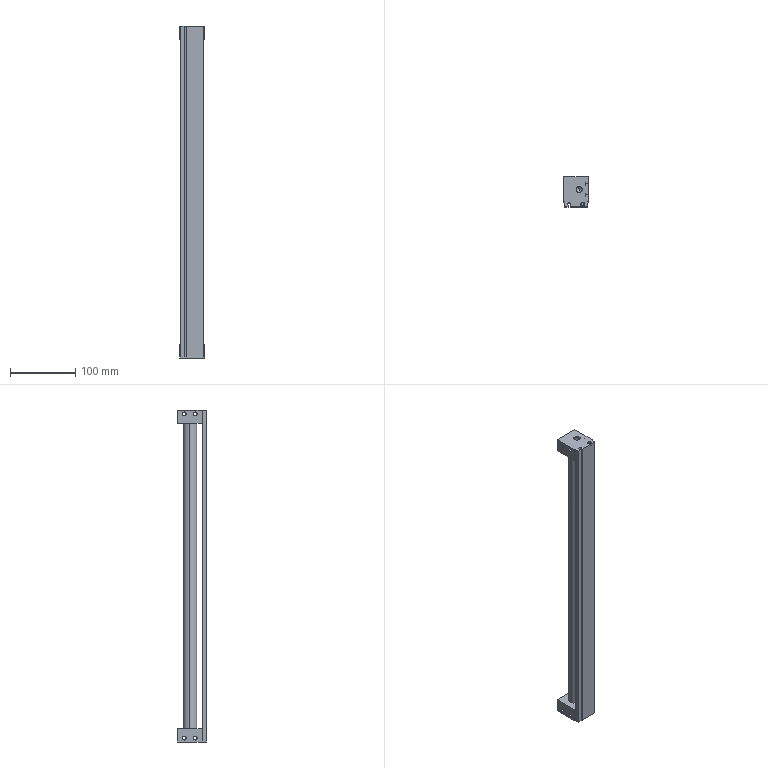Part | STEP file | 1_22 | 1 solid | 117 faces | box 38 x 45 x 507 mm | volume 342887 mm3 | plane 56 | cylinder 45 | cone 16 | commonest cylinder face diameters 4.917 x8 5.4 x8 9.5 x8 8.566 x4 9.228 x4 9.728 x4